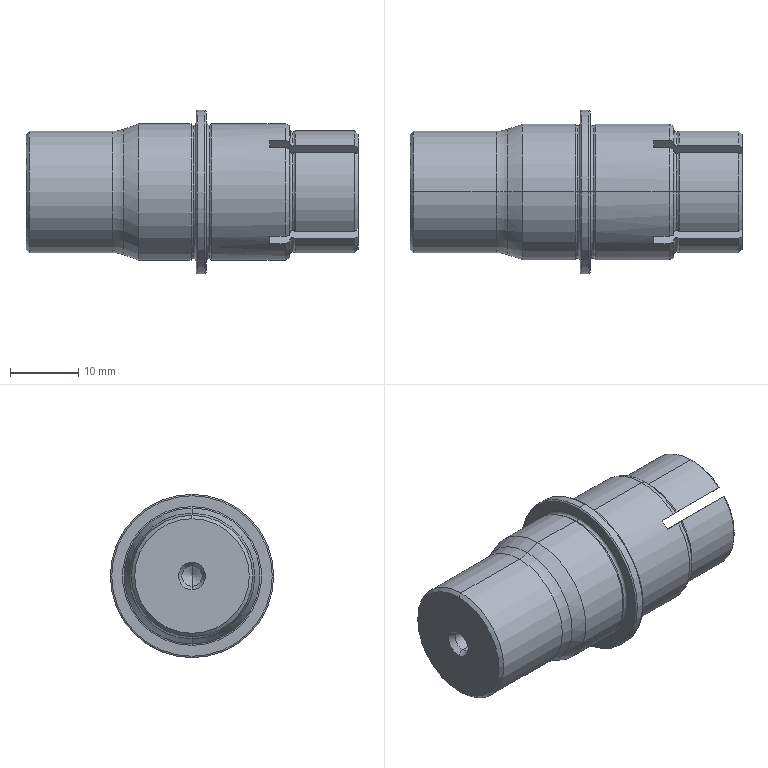Part | SolidWorks | features BaseBody 1 | 1 solid | 102 faces | box 48.8 x 24 x 24 mm | volume 9180 mm3 | cone 30 | torus 26 | plane 24 | cylinder 22 | commonest cylinder face diameters 14 x5 18 x5 20 x4 3 x2 14.5 x2 17.86 x2